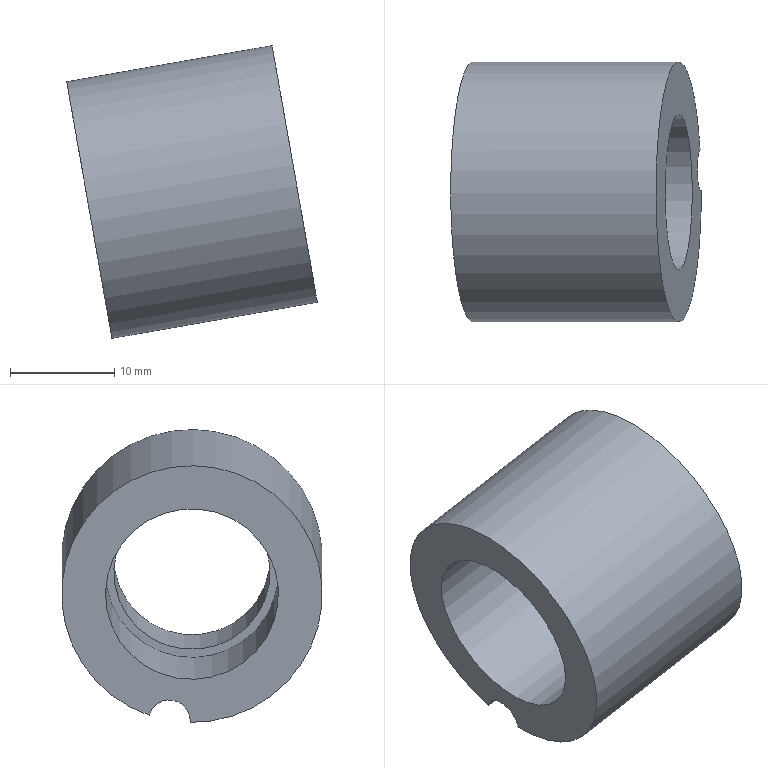Part | NX | features solid 2 | 1 solid | 7 faces | box 24.037 x 25 x 28.093 mm | volume 5685 mm3 | cylinder 4 | plane 3 | commonest cylinder face diameters 4 x1 15 x1 16.6 x1 25 x1
STEP:
#1=CARTESIAN_POINT('',(474.817,49.662,9.247));
#2=VERTEX_POINT('',#1);
#3=CARTESIAN_POINT('',(494.513,49.662,12.72));
#4=VERTEX_POINT('',#3);
#5=CARTESIAN_POINT('',(484.665,49.662,10.984));
#6=DIRECTION('',(0.9848,0.,0.1736));
#7=VECTOR('',#6,1000.);
#8=LINE('',#5,#7);
#9=EDGE_CURVE('',#2,#4,#8,.T.);
#10=ORIENTED_EDGE('',*,*,#9,.T.);
#11=CARTESIAN_POINT('',(494.393,53.589,13.402));
#12=VERTEX_POINT('',#11);
#13=CARTESIAN_POINT('',(492.343,49.483,25.029));
#14=DIRECTION('',(-0.9848,0.,-0.1736));
#15=DIRECTION('',(0.171,0.1736,-0.9698));
#16=AXIS2_PLACEMENT_3D('',#13,#14,#15);
#17=CIRCLE('',#16,12.5);
#18=EDGE_CURVE('',#4,#12,#17,.T.);
#19=ORIENTED_EDGE('',*,*,#18,.T.);
#20=CARTESIAN_POINT('',(474.697,53.589,9.929));
#21=VERTEX_POINT('',#20);
#22=CARTESIAN_POINT('',(484.545,53.589,11.666));
#23=DIRECTION('',(0.9848,0.,0.1736));
#24=VECTOR('',#23,1000.);
#25=LINE('',#22,#24);
#26=EDGE_CURVE('',#12,#21,#25,.F.);
#27=ORIENTED_EDGE('',*,*,#26,.T.);
#28=CARTESIAN_POINT('',(472.647,49.483,21.556));
#29=DIRECTION('',(-0.9848,0.,-0.1736));
#30=DIRECTION('',(0.171,0.1736,-0.9698));
#31=AXIS2_PLACEMENT_3D('',#28,#29,#30);
#32=CIRCLE('',#31,12.5);
#33=EDGE_CURVE('',#2,#21,#32,.T.);
#34=ORIENTED_EDGE('',*,*,#33,.F.);
#35=EDGE_LOOP('',(#10,#19,#27,#34));
#36=FACE_BOUND('',#35,.T.);
#37=CARTESIAN_POINT('',(472.647,49.483,21.556));
#38=DIRECTION('',(0.9848,0.,0.1736));
#39=DIRECTION('',(0.171,0.1736,-0.9698));
#40=AXIS2_PLACEMENT_3D('',#37,#38,#39);
#41=CYLINDRICAL_SURFACE('',#40,12.5);
#42=ADVANCED_FACE('',(#36),#41,.T.);
#43=CARTESIAN_POINT('',(474.066,50.924,13.506));
#44=VERTEX_POINT('',#43);
#45=CARTESIAN_POINT('',(472.647,49.483,21.556));
#46=DIRECTION('',(-0.9848,0.,-0.1736));
#47=DIRECTION('',(0.171,0.1736,-0.9698));
#48=AXIS2_PLACEMENT_3D('',#45,#46,#47);
#49=CIRCLE('',#48,8.3);
#50=EDGE_CURVE('',#44,#44,#49,.T.);
#51=ORIENTED_EDGE('',*,*,#50,.F.);
#52=EDGE_LOOP('',(#51));
#53=FACE_BOUND('',#52,.T.);
#54=ORIENTED_EDGE('',*,*,#33,.T.);
#55=CARTESIAN_POINT('',(474.784,51.653,9.433));
#56=DIRECTION('',(-0.9848,0.,-0.1736));
#57=DIRECTION('',(0.171,0.1736,-0.9698));
#58=AXIS2_PLACEMENT_3D('',#55,#56,#57);
#59=CIRCLE('',#58,2.);
#60=EDGE_CURVE('',#2,#21,#59,.T.);
#61=ORIENTED_EDGE('',*,*,#60,.F.);
#62=EDGE_LOOP('',(#54,#61));
#63=FACE_BOUND('',#62,.T.);
#64=CARTESIAN_POINT('',(472.647,49.483,21.556));
#65=DIRECTION('',(0.9848,0.,0.1736));
#66=DIRECTION('',(0.171,0.1736,-0.9698));
#67=AXIS2_PLACEMENT_3D('',#64,#65,#66);
#68=PLANE('',#67);
#69=ADVANCED_FACE('',(#53,#63),#68,.F.);
#70=CARTESIAN_POINT('',(491.04,49.483,32.415));
#71=VERTEX_POINT('',#70);
#72=CARTESIAN_POINT('',(492.343,49.483,25.029));
#73=DIRECTION('',(-0.9848,0.,-0.1736));
#74=DIRECTION('',(-0.1736,0.,0.9848));
#75=AXIS2_PLACEMENT_3D('',#72,#73,#74);
#76=CIRCLE('',#75,7.5);
#77=EDGE_CURVE('',#71,#71,#76,.T.);
#78=ORIENTED_EDGE('',*,*,#77,.T.);
#79=EDGE_LOOP('',(#78));
#80=FACE_BOUND('',#79,.T.);
#81=CARTESIAN_POINT('',(494.48,51.653,12.906));
#82=DIRECTION('',(-0.9848,0.,-0.1736));
#83=DIRECTION('',(0.171,0.1736,-0.9698));
#84=AXIS2_PLACEMENT_3D('',#81,#82,#83);
#85=CIRCLE('',#84,2.);
#86=EDGE_CURVE('',#4,#12,#85,.T.);
#87=ORIENTED_EDGE('',*,*,#86,.T.);
#88=ORIENTED_EDGE('',*,*,#18,.F.);
#89=EDGE_LOOP('',(#87,#88));
#90=FACE_BOUND('',#89,.T.);
#91=CARTESIAN_POINT('',(492.343,49.483,25.029));
#92=DIRECTION('',(0.9848,0.,0.1736));
#93=DIRECTION('',(0.171,0.1736,-0.9698));
#94=AXIS2_PLACEMENT_3D('',#91,#92,#93);
#95=PLANE('',#94);
#96=ADVANCED_FACE('',(#80,#90),#95,.T.);
#97=ORIENTED_EDGE('',*,*,#50,.T.);
#98=EDGE_LOOP('',(#97));
#99=FACE_BOUND('',#98,.T.);
#100=CARTESIAN_POINT('',(485.884,50.924,15.59));
#101=VERTEX_POINT('',#100);
#102=CARTESIAN_POINT('',(484.464,49.483,23.64));
#103=DIRECTION('',(-0.9848,0.,-0.1736));
#104=DIRECTION('',(0.171,0.1736,-0.9698));
#105=AXIS2_PLACEMENT_3D('',#102,#103,#104);
#106=CIRCLE('',#105,8.3);
#107=EDGE_CURVE('',#101,#101,#106,.T.);
#108=ORIENTED_EDGE('',*,*,#107,.F.);
#109=EDGE_LOOP('',(#108));
#110=FACE_BOUND('',#109,.T.);
#111=CARTESIAN_POINT('',(472.647,49.483,21.556));
#112=DIRECTION('',(0.9848,0.,0.1736));
#113=DIRECTION('',(0.171,0.1736,-0.9698));
#114=AXIS2_PLACEMENT_3D('',#111,#112,#113);
#115=CYLINDRICAL_SURFACE('',#114,8.3);
#116=ADVANCED_FACE('',(#99,#110),#115,.F.);
#117=CARTESIAN_POINT('',(483.162,49.483,31.026));
#118=VERTEX_POINT('',#117);
#119=CARTESIAN_POINT('',(484.464,49.483,23.64));
#120=DIRECTION('',(-0.9848,0.,-0.1736));
#121=DIRECTION('',(-0.1736,0.,0.9848));
#122=AXIS2_PLACEMENT_3D('',#119,#120,#121);
#123=CIRCLE('',#122,7.5);
#124=EDGE_CURVE('',#118,#118,#123,.T.);
#125=ORIENTED_EDGE('',*,*,#124,.F.);
#126=EDGE_LOOP('',(#125));
#127=FACE_BOUND('',#126,.T.);
#128=ORIENTED_EDGE('',*,*,#107,.T.);
#129=EDGE_LOOP('',(#128));
#130=FACE_BOUND('',#129,.T.);
#131=CARTESIAN_POINT('',(484.464,49.483,23.64));
#132=DIRECTION('',(0.9848,0.,0.1736));
#133=DIRECTION('',(0.171,0.1736,-0.9698));
#134=AXIS2_PLACEMENT_3D('',#131,#132,#133);
#135=PLANE('',#134);
#136=ADVANCED_FACE('',(#127,#130),#135,.F.);
#137=ORIENTED_EDGE('',*,*,#9,.F.);
#138=ORIENTED_EDGE('',*,*,#60,.T.);
#139=ORIENTED_EDGE('',*,*,#26,.F.);
#140=ORIENTED_EDGE('',*,*,#86,.F.);
#141=EDGE_LOOP('',(#137,#138,#139,#140));
#142=FACE_BOUND('',#141,.T.);
#143=CARTESIAN_POINT('',(474.784,51.653,9.433));
#144=DIRECTION('',(0.9848,0.,0.1736));
#145=DIRECTION('',(0.171,0.1736,-0.9698));
#146=AXIS2_PLACEMENT_3D('',#143,#144,#145);
#147=CYLINDRICAL_SURFACE('',#146,2.);
#148=ADVANCED_FACE('',(#142),#147,.F.);
#149=ORIENTED_EDGE('',*,*,#77,.F.);
#150=EDGE_LOOP('',(#149));
#151=FACE_BOUND('',#150,.T.);
#152=ORIENTED_EDGE('',*,*,#124,.T.);
#153=EDGE_LOOP('',(#152));
#154=FACE_BOUND('',#153,.T.);
#155=CARTESIAN_POINT('',(472.647,49.483,21.556));
#156=DIRECTION('',(0.9848,0.,0.1736));
#157=DIRECTION('',(0.171,0.1736,-0.9698));
#158=AXIS2_PLACEMENT_3D('',#155,#156,#157);
#159=CYLINDRICAL_SURFACE('',#158,7.5);
#160=ADVANCED_FACE('',(#151,#154),#159,.F.);
#161=CLOSED_SHELL('',(#42,#69,#96,#116,#136,#148,#160));
#162=MANIFOLD_SOLID_BREP('',#161);
#163=(LENGTH_UNIT()NAMED_UNIT(*)SI_UNIT(.MILLI.,.METRE.));
#164=UNCERTAINTY_MEASURE_WITH_UNIT(LENGTH_MEASURE(0.00001),#163,'','');
#165=(NAMED_UNIT(*)PLANE_ANGLE_UNIT()SI_UNIT($,.RADIAN.));
#166=(NAMED_UNIT(*)SI_UNIT($,.STERADIAN.)SOLID_ANGLE_UNIT());
#167=(GEOMETRIC_REPRESENTATION_CONTEXT(3)GLOBAL_UNCERTAINTY_ASSIGNED_CONTEXT((#164))GLOBAL_UNIT_ASSIGNED_CONTEXT((#163,#165,#166))REPRESENTATION_CONTEXT('',''));
#168=ADVANCED_BREP_SHAPE_REPRESENTATION('',(#162),#167);